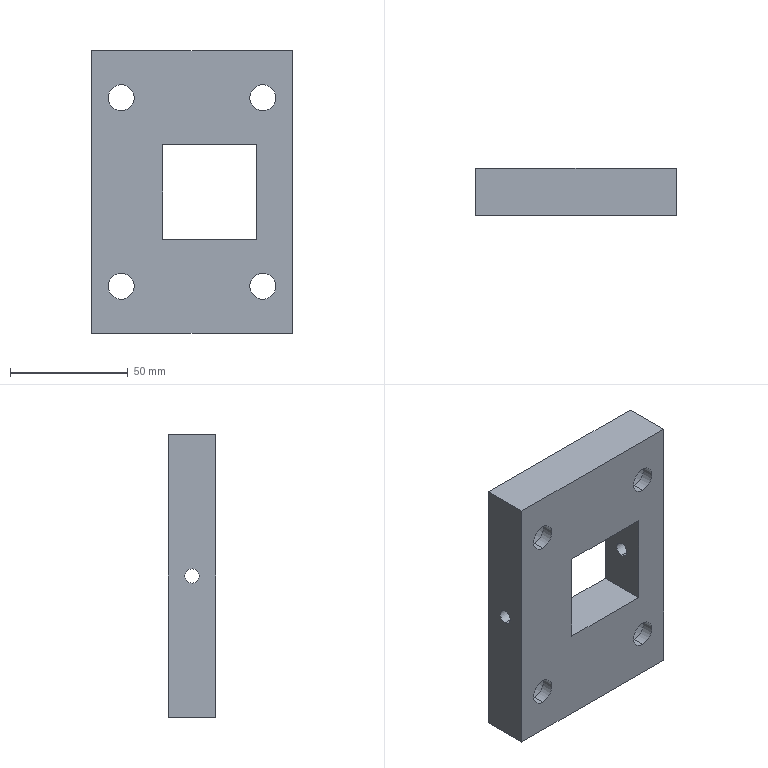Part | SolidWorks | features ICE 2, Extrusion 1 | 1 solid | 34 faces | box 85 x 20 x 120 mm | volume 147044 mm3 | cylinder 20 | plane 14 | commonest cylinder face diameters 11 x8 21.5 x8 6 x4
STEP:
#1=CARTESIAN_POINT('',(42.5,10.,-3.));
#2=VERTEX_POINT('',#1);
#3=CARTESIAN_POINT('',(42.5,10.,3.));
#4=VERTEX_POINT('',#3);
#5=CARTESIAN_POINT('',(42.5,10.,0.));
#6=DIRECTION('',(-1.,0.,0.));
#7=DIRECTION('',(0.,0.,1.));
#8=AXIS2_PLACEMENT_3D('',#5,#6,#7);
#9=CIRCLE('',#8,3.);
#10=EDGE_CURVE('',#2,#4,#9,.T.);
#11=ORIENTED_EDGE('',*,*,#10,.F.);
#12=CARTESIAN_POINT('',(27.5,10.,-3.));
#13=VERTEX_POINT('',#12);
#14=CARTESIAN_POINT('',(42.5,10.,-3.));
#15=DIRECTION('',(-1.,0.,0.));
#16=VECTOR('',#15,1000.);
#17=LINE('',#14,#16);
#18=EDGE_CURVE('',#2,#13,#17,.T.);
#19=ORIENTED_EDGE('',*,*,#18,.T.);
#20=CARTESIAN_POINT('',(27.5,10.,3.));
#21=VERTEX_POINT('',#20);
#22=CARTESIAN_POINT('',(27.5,10.,0.));
#23=DIRECTION('',(-1.,0.,0.));
#24=DIRECTION('',(0.,0.,1.));
#25=AXIS2_PLACEMENT_3D('',#22,#23,#24);
#26=CIRCLE('',#25,3.);
#27=EDGE_CURVE('',#13,#21,#26,.T.);
#28=ORIENTED_EDGE('',*,*,#27,.T.);
#29=CARTESIAN_POINT('',(42.5,10.,3.));
#30=DIRECTION('',(-1.,0.,0.));
#31=VECTOR('',#30,1000.);
#32=LINE('',#29,#31);
#33=EDGE_CURVE('',#4,#21,#32,.T.);
#34=ORIENTED_EDGE('',*,*,#33,.F.);
#35=EDGE_LOOP('',(#11,#19,#28,#34));
#36=FACE_OUTER_BOUND('',#35,.T.);
#37=CARTESIAN_POINT('',(42.5,10.,0.));
#38=DIRECTION('',(-1.,0.,0.));
#39=DIRECTION('',(0.,0.,1.));
#40=AXIS2_PLACEMENT_3D('',#37,#38,#39);
#41=CYLINDRICAL_SURFACE('',#40,3.);
#42=ADVANCED_FACE('',(#36),#41,.F.);
#43=CARTESIAN_POINT('',(-12.5,10.,3.));
#44=VERTEX_POINT('',#43);
#45=CARTESIAN_POINT('',(-12.5,10.,-3.));
#46=VERTEX_POINT('',#45);
#47=CARTESIAN_POINT('',(-12.5,10.,0.));
#48=DIRECTION('',(1.,0.,0.));
#49=DIRECTION('',(0.,0.,-1.));
#50=AXIS2_PLACEMENT_3D('',#47,#48,#49);
#51=CIRCLE('',#50,3.);
#52=EDGE_CURVE('',#44,#46,#51,.T.);
#53=ORIENTED_EDGE('',*,*,#52,.T.);
#54=CARTESIAN_POINT('',(-42.5,10.,-3.));
#55=VERTEX_POINT('',#54);
#56=CARTESIAN_POINT('',(42.5,10.,-3.));
#57=DIRECTION('',(-1.,0.,0.));
#58=VECTOR('',#57,1000.);
#59=LINE('',#56,#58);
#60=EDGE_CURVE('',#46,#55,#59,.T.);
#61=ORIENTED_EDGE('',*,*,#60,.T.);
#62=CARTESIAN_POINT('',(-42.5,10.,3.));
#63=VERTEX_POINT('',#62);
#64=CARTESIAN_POINT('',(-42.5,10.,0.));
#65=DIRECTION('',(-1.,0.,0.));
#66=DIRECTION('',(0.,0.,1.));
#67=AXIS2_PLACEMENT_3D('',#64,#65,#66);
#68=CIRCLE('',#67,3.);
#69=EDGE_CURVE('',#55,#63,#68,.T.);
#70=ORIENTED_EDGE('',*,*,#69,.T.);
#71=CARTESIAN_POINT('',(42.5,10.,3.));
#72=DIRECTION('',(-1.,0.,0.));
#73=VECTOR('',#72,1000.);
#74=LINE('',#71,#73);
#75=EDGE_CURVE('',#44,#63,#74,.T.);
#76=ORIENTED_EDGE('',*,*,#75,.F.);
#77=EDGE_LOOP('',(#53,#61,#70,#76));
#78=FACE_OUTER_BOUND('',#77,.T.);
#79=CARTESIAN_POINT('',(42.5,10.,0.));
#80=DIRECTION('',(-1.,0.,0.));
#81=DIRECTION('',(0.,0.,1.));
#82=AXIS2_PLACEMENT_3D('',#79,#80,#81);
#83=CYLINDRICAL_SURFACE('',#82,3.);
#84=ADVANCED_FACE('',(#78),#83,.F.);
#85=CARTESIAN_POINT('',(-30.,5.,-50.75));
#86=VERTEX_POINT('',#85);
#87=CARTESIAN_POINT('',(-30.,5.,-29.25));
#88=VERTEX_POINT('',#87);
#89=CARTESIAN_POINT('',(-30.,5.,-40.));
#90=DIRECTION('',(0.,1.,0.));
#91=DIRECTION('',(0.,0.,1.));
#92=AXIS2_PLACEMENT_3D('',#89,#90,#91);
#93=CIRCLE('',#92,10.75);
#94=EDGE_CURVE('',#86,#88,#93,.T.);
#95=ORIENTED_EDGE('',*,*,#94,.F.);
#96=CARTESIAN_POINT('',(-30.,20.,-50.75));
#97=VERTEX_POINT('',#96);
#98=CARTESIAN_POINT('',(-30.,5.,-50.75));
#99=DIRECTION('',(0.,1.,0.));
#100=VECTOR('',#99,1000.);
#101=LINE('',#98,#100);
#102=EDGE_CURVE('',#86,#97,#101,.T.);
#103=ORIENTED_EDGE('',*,*,#102,.T.);
#104=CARTESIAN_POINT('',(-30.,20.,-29.25));
#105=VERTEX_POINT('',#104);
#106=CARTESIAN_POINT('',(-30.,20.,-40.));
#107=DIRECTION('',(0.,1.,0.));
#108=DIRECTION('',(0.,0.,1.));
#109=AXIS2_PLACEMENT_3D('',#106,#107,#108);
#110=CIRCLE('',#109,10.75);
#111=EDGE_CURVE('',#97,#105,#110,.T.);
#112=ORIENTED_EDGE('',*,*,#111,.T.);
#113=CARTESIAN_POINT('',(-30.,5.,-29.25));
#114=DIRECTION('',(0.,1.,0.));
#115=VECTOR('',#114,1000.);
#116=LINE('',#113,#115);
#117=EDGE_CURVE('',#88,#105,#116,.T.);
#118=ORIENTED_EDGE('',*,*,#117,.F.);
#119=EDGE_LOOP('',(#95,#103,#112,#118));
#120=FACE_OUTER_BOUND('',#119,.T.);
#121=CARTESIAN_POINT('',(-30.,5.,-40.));
#122=DIRECTION('',(0.,1.,0.));
#123=DIRECTION('',(0.,0.,1.));
#124=AXIS2_PLACEMENT_3D('',#121,#122,#123);
#125=CYLINDRICAL_SURFACE('',#124,10.75);
#126=ADVANCED_FACE('',(#120),#125,.F.);
#127=CARTESIAN_POINT('',(30.,5.,-50.75));
#128=VERTEX_POINT('',#127);
#129=CARTESIAN_POINT('',(30.,5.,-29.25));
#130=VERTEX_POINT('',#129);
#131=CARTESIAN_POINT('',(30.,5.,-40.));
#132=DIRECTION('',(0.,1.,0.));
#133=DIRECTION('',(0.,0.,1.));
#134=AXIS2_PLACEMENT_3D('',#131,#132,#133);
#135=CIRCLE('',#134,10.75);
#136=EDGE_CURVE('',#128,#130,#135,.T.);
#137=ORIENTED_EDGE('',*,*,#136,.F.);
#138=CARTESIAN_POINT('',(30.,20.,-50.75));
#139=VERTEX_POINT('',#138);
#140=CARTESIAN_POINT('',(30.,5.,-50.75));
#141=DIRECTION('',(0.,1.,0.));
#142=VECTOR('',#141,1000.);
#143=LINE('',#140,#142);
#144=EDGE_CURVE('',#128,#139,#143,.T.);
#145=ORIENTED_EDGE('',*,*,#144,.T.);
#146=CARTESIAN_POINT('',(30.,20.,-29.25));
#147=VERTEX_POINT('',#146);
#148=CARTESIAN_POINT('',(30.,20.,-40.));
#149=DIRECTION('',(0.,1.,0.));
#150=DIRECTION('',(0.,0.,1.));
#151=AXIS2_PLACEMENT_3D('',#148,#149,#150);
#152=CIRCLE('',#151,10.75);
#153=EDGE_CURVE('',#139,#147,#152,.T.);
#154=ORIENTED_EDGE('',*,*,#153,.T.);
#155=CARTESIAN_POINT('',(30.,5.,-29.25));
#156=DIRECTION('',(0.,1.,0.));
#157=VECTOR('',#156,1000.);
#158=LINE('',#155,#157);
#159=EDGE_CURVE('',#130,#147,#158,.T.);
#160=ORIENTED_EDGE('',*,*,#159,.F.);
#161=EDGE_LOOP('',(#137,#145,#154,#160));
#162=FACE_OUTER_BOUND('',#161,.T.);
#163=CARTESIAN_POINT('',(30.,5.,-40.));
#164=DIRECTION('',(0.,1.,0.));
#165=DIRECTION('',(0.,0.,1.));
#166=AXIS2_PLACEMENT_3D('',#163,#164,#165);
#167=CYLINDRICAL_SURFACE('',#166,10.75);
#168=ADVANCED_FACE('',(#162),#167,.F.);
#169=CARTESIAN_POINT('',(30.,5.,29.25));
#170=VERTEX_POINT('',#169);
#171=CARTESIAN_POINT('',(30.,5.,50.75));
#172=VERTEX_POINT('',#171);
#173=CARTESIAN_POINT('',(30.,5.,40.));
#174=DIRECTION('',(0.,1.,0.));
#175=DIRECTION('',(0.,0.,1.));
#176=AXIS2_PLACEMENT_3D('',#173,#174,#175);
#177=CIRCLE('',#176,10.75);
#178=EDGE_CURVE('',#170,#172,#177,.T.);
#179=ORIENTED_EDGE('',*,*,#178,.F.);
#180=CARTESIAN_POINT('',(30.,20.,29.25));
#181=VERTEX_POINT('',#180);
#182=CARTESIAN_POINT('',(30.,5.,29.25));
#183=DIRECTION('',(0.,1.,0.));
#184=VECTOR('',#183,1000.);
#185=LINE('',#182,#184);
#186=EDGE_CURVE('',#170,#181,#185,.T.);
#187=ORIENTED_EDGE('',*,*,#186,.T.);
#188=CARTESIAN_POINT('',(30.,20.,50.75));
#189=VERTEX_POINT('',#188);
#190=CARTESIAN_POINT('',(30.,20.,40.));
#191=DIRECTION('',(0.,1.,0.));
#192=DIRECTION('',(0.,0.,1.));
#193=AXIS2_PLACEMENT_3D('',#190,#191,#192);
#194=CIRCLE('',#193,10.75);
#195=EDGE_CURVE('',#181,#189,#194,.T.);
#196=ORIENTED_EDGE('',*,*,#195,.T.);
#197=CARTESIAN_POINT('',(30.,5.,50.75));
#198=DIRECTION('',(0.,1.,0.));
#199=VECTOR('',#198,1000.);
#200=LINE('',#197,#199);
#201=EDGE_CURVE('',#172,#189,#200,.T.);
#202=ORIENTED_EDGE('',*,*,#201,.F.);
#203=EDGE_LOOP('',(#179,#187,#196,#202));
#204=FACE_OUTER_BOUND('',#203,.T.);
#205=CARTESIAN_POINT('',(30.,5.,40.));
#206=DIRECTION('',(0.,1.,0.));
#207=DIRECTION('',(0.,0.,1.));
#208=AXIS2_PLACEMENT_3D('',#205,#206,#207);
#209=CYLINDRICAL_SURFACE('',#208,10.75);
#210=ADVANCED_FACE('',(#204),#209,.F.);
#211=CARTESIAN_POINT('',(-30.,5.,29.25));
#212=VERTEX_POINT('',#211);
#213=CARTESIAN_POINT('',(-30.,5.,50.75));
#214=VERTEX_POINT('',#213);
#215=CARTESIAN_POINT('',(-30.,5.,40.));
#216=DIRECTION('',(0.,1.,0.));
#217=DIRECTION('',(0.,0.,1.));
#218=AXIS2_PLACEMENT_3D('',#215,#216,#217);
#219=CIRCLE('',#218,10.75);
#220=EDGE_CURVE('',#212,#214,#219,.T.);
#221=ORIENTED_EDGE('',*,*,#220,.F.);
#222=CARTESIAN_POINT('',(-30.,20.,29.25));
#223=VERTEX_POINT('',#222);
#224=CARTESIAN_POINT('',(-30.,5.,29.25));
#225=DIRECTION('',(0.,1.,0.));
#226=VECTOR('',#225,1000.);
#227=LINE('',#224,#226);
#228=EDGE_CURVE('',#212,#223,#227,.T.);
#229=ORIENTED_EDGE('',*,*,#228,.T.);
#230=CARTESIAN_POINT('',(-30.,20.,50.75));
#231=VERTEX_POINT('',#230);
#232=CARTESIAN_POINT('',(-30.,20.,40.));
#233=DIRECTION('',(0.,1.,0.));
#234=DIRECTION('',(0.,0.,1.));
#235=AXIS2_PLACEMENT_3D('',#232,#233,#234);
#236=CIRCLE('',#235,10.75);
#237=EDGE_CURVE('',#223,#231,#236,.T.);
#238=ORIENTED_EDGE('',*,*,#237,.T.);
#239=CARTESIAN_POINT('',(-30.,5.,50.75));
#240=DIRECTION('',(0.,1.,0.));
#241=VECTOR('',#240,1000.);
#242=LINE('',#239,#241);
#243=EDGE_CURVE('',#214,#231,#242,.T.);
#244=ORIENTED_EDGE('',*,*,#243,.F.);
#245=EDGE_LOOP('',(#221,#229,#238,#244));
#246=FACE_OUTER_BOUND('',#245,.T.);
#247=CARTESIAN_POINT('',(-30.,5.,40.));
#248=DIRECTION('',(0.,1.,0.));
#249=DIRECTION('',(0.,0.,1.));
#250=AXIS2_PLACEMENT_3D('',#247,#248,#249);
#251=CYLINDRICAL_SURFACE('',#250,10.75);
#252=ADVANCED_FACE('',(#246),#251,.F.);
#253=CARTESIAN_POINT('',(-30.,5.,34.5));
#254=VERTEX_POINT('',#253);
#255=CARTESIAN_POINT('',(-30.,5.,45.5));
#256=VERTEX_POINT('',#255);
#257=CARTESIAN_POINT('',(-30.,5.,40.));
#258=DIRECTION('',(0.,1.,0.));
#259=DIRECTION('',(0.,0.,1.));
#260=AXIS2_PLACEMENT_3D('',#257,#258,#259);
#261=CIRCLE('',#260,5.5);
#262=EDGE_CURVE('',#254,#256,#261,.T.);
#263=ORIENTED_EDGE('',*,*,#262,.T.);
#264=CARTESIAN_POINT('',(-30.,0.,45.5));
#265=VERTEX_POINT('',#264);
#266=CARTESIAN_POINT('',(-30.,20.,45.5));
#267=DIRECTION('',(0.,-1.,0.));
#268=VECTOR('',#267,1000.);
#269=LINE('',#266,#268);
#270=EDGE_CURVE('',#256,#265,#269,.T.);
#271=ORIENTED_EDGE('',*,*,#270,.T.);
#272=CARTESIAN_POINT('',(-30.,0.,34.5));
#273=VERTEX_POINT('',#272);
#274=CARTESIAN_POINT('',(-30.,0.,40.));
#275=DIRECTION('',(0.,1.,0.));
#276=DIRECTION('',(0.,0.,1.));
#277=AXIS2_PLACEMENT_3D('',#274,#275,#276);
#278=CIRCLE('',#277,5.5);
#279=EDGE_CURVE('',#273,#265,#278,.T.);
#280=ORIENTED_EDGE('',*,*,#279,.F.);
#281=CARTESIAN_POINT('',(-30.,20.,34.5));
#282=DIRECTION('',(0.,-1.,0.));
#283=VECTOR('',#282,1000.);
#284=LINE('',#281,#283);
#285=EDGE_CURVE('',#254,#273,#284,.T.);
#286=ORIENTED_EDGE('',*,*,#285,.F.);
#287=EDGE_LOOP('',(#263,#271,#280,#286));
#288=FACE_OUTER_BOUND('',#287,.T.);
#289=CARTESIAN_POINT('',(-30.,20.,40.));
#290=DIRECTION('',(0.,-1.,0.));
#291=DIRECTION('',(0.,0.,-1.));
#292=AXIS2_PLACEMENT_3D('',#289,#290,#291);
#293=CYLINDRICAL_SURFACE('',#292,5.5);
#294=ADVANCED_FACE('',(#288),#293,.F.);
#295=CARTESIAN_POINT('',(30.,5.,34.5));
#296=VERTEX_POINT('',#295);
#297=CARTESIAN_POINT('',(30.,5.,45.5));
#298=VERTEX_POINT('',#297);
#299=CARTESIAN_POINT('',(30.,5.,40.));
#300=DIRECTION('',(0.,1.,0.));
#301=DIRECTION('',(0.,0.,1.));
#302=AXIS2_PLACEMENT_3D('',#299,#300,#301);
#303=CIRCLE('',#302,5.5);
#304=EDGE_CURVE('',#296,#298,#303,.T.);
#305=ORIENTED_EDGE('',*,*,#304,.T.);
#306=CARTESIAN_POINT('',(30.,0.,45.5));
#307=VERTEX_POINT('',#306);
#308=CARTESIAN_POINT('',(30.,20.,45.5));
#309=DIRECTION('',(0.,-1.,0.));
#310=VECTOR('',#309,1000.);
#311=LINE('',#308,#310);
#312=EDGE_CURVE('',#298,#307,#311,.T.);
#313=ORIENTED_EDGE('',*,*,#312,.T.);
#314=CARTESIAN_POINT('',(30.,0.,34.5));
#315=VERTEX_POINT('',#314);
#316=CARTESIAN_POINT('',(30.,0.,40.));
#317=DIRECTION('',(0.,1.,0.));
#318=DIRECTION('',(0.,0.,1.));
#319=AXIS2_PLACEMENT_3D('',#316,#317,#318);
#320=CIRCLE('',#319,5.5);
#321=EDGE_CURVE('',#315,#307,#320,.T.);
#322=ORIENTED_EDGE('',*,*,#321,.F.);
#323=CARTESIAN_POINT('',(30.,20.,34.5));
#324=DIRECTION('',(0.,-1.,0.));
#325=VECTOR('',#324,1000.);
#326=LINE('',#323,#325);
#327=EDGE_CURVE('',#296,#315,#326,.T.);
#328=ORIENTED_EDGE('',*,*,#327,.F.);
#329=EDGE_LOOP('',(#305,#313,#322,#328));
#330=FACE_OUTER_BOUND('',#329,.T.);
#331=CARTESIAN_POINT('',(30.,20.,40.));
#332=DIRECTION('',(0.,-1.,0.));
#333=DIRECTION('',(0.,0.,-1.));
#334=AXIS2_PLACEMENT_3D('',#331,#332,#333);
#335=CYLINDRICAL_SURFACE('',#334,5.5);
#336=ADVANCED_FACE('',(#330),#335,.F.);
#337=CARTESIAN_POINT('',(30.,5.,-45.5));
#338=VERTEX_POINT('',#337);
#339=CARTESIAN_POINT('',(30.,5.,-34.5));
#340=VERTEX_POINT('',#339);
#341=CARTESIAN_POINT('',(30.,5.,-40.));
#342=DIRECTION('',(0.,1.,0.));
#343=DIRECTION('',(0.,0.,1.));
#344=AXIS2_PLACEMENT_3D('',#341,#342,#343);
#345=CIRCLE('',#344,5.5);
#346=EDGE_CURVE('',#338,#340,#345,.T.);
#347=ORIENTED_EDGE('',*,*,#346,.T.);
#348=CARTESIAN_POINT('',(30.,0.,-34.5));
#349=VERTEX_POINT('',#348);
#350=CARTESIAN_POINT('',(30.,20.,-34.5));
#351=DIRECTION('',(0.,-1.,0.));
#352=VECTOR('',#351,1000.);
#353=LINE('',#350,#352);
#354=EDGE_CURVE('',#340,#349,#353,.T.);
#355=ORIENTED_EDGE('',*,*,#354,.T.);
#356=CARTESIAN_POINT('',(30.,0.,-45.5));
#357=VERTEX_POINT('',#356);
#358=CARTESIAN_POINT('',(30.,0.,-40.));
#359=DIRECTION('',(0.,1.,0.));
#360=DIRECTION('',(0.,0.,1.));
#361=AXIS2_PLACEMENT_3D('',#358,#359,#360);
#362=CIRCLE('',#361,5.5);
#363=EDGE_CURVE('',#357,#349,#362,.T.);
#364=ORIENTED_EDGE('',*,*,#363,.F.);
#365=CARTESIAN_POINT('',(30.,20.,-45.5));
#366=DIRECTION('',(0.,-1.,0.));
#367=VECTOR('',#366,1000.);
#368=LINE('',#365,#367);
#369=EDGE_CURVE('',#338,#357,#368,.T.);
#370=ORIENTED_EDGE('',*,*,#369,.F.);
#371=EDGE_LOOP('',(#347,#355,#364,#370));
#372=FACE_OUTER_BOUND('',#371,.T.);
#373=CARTESIAN_POINT('',(30.,20.,-40.));
#374=DIRECTION('',(0.,-1.,0.));
#375=DIRECTION('',(0.,0.,-1.));
#376=AXIS2_PLACEMENT_3D('',#373,#374,#375);
#377=CYLINDRICAL_SURFACE('',#376,5.5);
#378=ADVANCED_FACE('',(#372),#377,.F.);
#379=CARTESIAN_POINT('',(-30.,5.,-45.5));
#380=VERTEX_POINT('',#379);
#381=CARTESIAN_POINT('',(-30.,5.,-34.5));
#382=VERTEX_POINT('',#381);
#383=CARTESIAN_POINT('',(-30.,5.,-40.));
#384=DIRECTION('',(0.,1.,0.));
#385=DIRECTION('',(0.,0.,1.));
#386=AXIS2_PLACEMENT_3D('',#383,#384,#385);
#387=CIRCLE('',#386,5.5);
#388=EDGE_CURVE('',#380,#382,#387,.T.);
#389=ORIENTED_EDGE('',*,*,#388,.T.);
#390=CARTESIAN_POINT('',(-30.,0.,-34.5));
#391=VERTEX_POINT('',#390);
#392=CARTESIAN_POINT('',(-30.,20.,-34.5));
#393=DIRECTION('',(0.,-1.,0.));
#394=VECTOR('',#393,1000.);
#395=LINE('',#392,#394);
#396=EDGE_CURVE('',#382,#391,#395,.T.);
#397=ORIENTED_EDGE('',*,*,#396,.T.);
#398=CARTESIAN_POINT('',(-30.,0.,-45.5));
#399=VERTEX_POINT('',#398);
#400=CARTESIAN_POINT('',(-30.,0.,-40.));
#401=DIRECTION('',(0.,1.,0.));
#402=DIRECTION('',(0.,0.,1.));
#403=AXIS2_PLACEMENT_3D('',#400,#401,#402);
#404=CIRCLE('',#403,5.5);
#405=EDGE_CURVE('',#399,#391,#404,.T.);
#406=ORIENTED_EDGE('',*,*,#405,.F.);
#407=CARTESIAN_POINT('',(-30.,20.,-45.5));
#408=DIRECTION('',(0.,-1.,0.));
#409=VECTOR('',#408,1000.);
#410=LINE('',#407,#409);
#411=EDGE_CURVE('',#380,#399,#410,.T.);
#412=ORIENTED_EDGE('',*,*,#411,.F.);
#413=EDGE_LOOP('',(#389,#397,#406,#412));
#414=FACE_OUTER_BOUND('',#413,.T.);
#415=CARTESIAN_POINT('',(-30.,20.,-40.));
#416=DIRECTION('',(0.,-1.,0.));
#417=DIRECTION('',(0.,0.,-1.));
#418=AXIS2_PLACEMENT_3D('',#415,#416,#417);
#419=CYLINDRICAL_SURFACE('',#418,5.5);
#420=ADVANCED_FACE('',(#414),#419,.F.);
#421=ORIENTED_EDGE('',*,*,#396,.F.);
#422=CARTESIAN_POINT('',(-30.,5.,-40.));
#423=DIRECTION('',(0.,1.,0.));
#424=DIRECTION('',(0.,0.,1.));
#425=AXIS2_PLACEMENT_3D('',#422,#423,#424);
#426=CIRCLE('',#425,5.5);
#427=EDGE_CURVE('',#382,#380,#426,.T.);
#428=ORIENTED_EDGE('',*,*,#427,.T.);
#429=ORIENTED_EDGE('',*,*,#411,.T.);
#430=CARTESIAN_POINT('',(-30.,0.,-40.));
#431=DIRECTION('',(0.,1.,0.));
#432=DIRECTION('',(0.,0.,1.));
#433=AXIS2_PLACEMENT_3D('',#430,#431,#432);
#434=CIRCLE('',#433,5.5);
#435=EDGE_CURVE('',#391,#399,#434,.T.);
#436=ORIENTED_EDGE('',*,*,#435,.F.);
#437=EDGE_LOOP('',(#421,#428,#429,#436));
#438=FACE_OUTER_BOUND('',#437,.T.);
#439=CARTESIAN_POINT('',(-30.,20.,-40.));
#440=DIRECTION('',(0.,-1.,0.));
#441=DIRECTION('',(0.,0.,-1.));
#442=AXIS2_PLACEMENT_3D('',#439,#440,#441);
#443=CYLINDRICAL_SURFACE('',#442,5.5);
#444=ADVANCED_FACE('',(#438),#443,.F.);
#445=ORIENTED_EDGE('',*,*,#354,.F.);
#446=CARTESIAN_POINT('',(30.,5.,-40.));
#447=DIRECTION('',(0.,1.,0.));
#448=DIRECTION('',(0.,0.,1.));
#449=AXIS2_PLACEMENT_3D('',#446,#447,#448);
#450=CIRCLE('',#449,5.5);
#451=EDGE_CURVE('',#340,#338,#450,.T.);
#452=ORIENTED_EDGE('',*,*,#451,.T.);
#453=ORIENTED_EDGE('',*,*,#369,.T.);
#454=CARTESIAN_POINT('',(30.,0.,-40.));
#455=DIRECTION('',(0.,1.,0.));
#456=DIRECTION('',(0.,0.,1.));
#457=AXIS2_PLACEMENT_3D('',#454,#455,#456);
#458=CIRCLE('',#457,5.5);
#459=EDGE_CURVE('',#349,#357,#458,.T.);
#460=ORIENTED_EDGE('',*,*,#459,.F.);
#461=EDGE_LOOP('',(#445,#452,#453,#460));
#462=FACE_OUTER_BOUND('',#461,.T.);
#463=CARTESIAN_POINT('',(30.,20.,-40.));
#464=DIRECTION('',(0.,-1.,0.));
#465=DIRECTION('',(0.,0.,-1.));
#466=AXIS2_PLACEMENT_3D('',#463,#464,#465);
#467=CYLINDRICAL_SURFACE('',#466,5.5);
#468=ADVANCED_FACE('',(#462),#467,.F.);
#469=ORIENTED_EDGE('',*,*,#312,.F.);
#470=CARTESIAN_POINT('',(30.,5.,40.));
#471=DIRECTION('',(0.,1.,0.));
#472=DIRECTION('',(0.,0.,1.));
#473=AXIS2_PLACEMENT_3D('',#470,#471,#472);
#474=CIRCLE('',#473,5.5);
#475=EDGE_CURVE('',#298,#296,#474,.T.);
#476=ORIENTED_EDGE('',*,*,#475,.T.);
#477=ORIENTED_EDGE('',*,*,#327,.T.);
#478=CARTESIAN_POINT('',(30.,0.,40.));
#479=DIRECTION('',(0.,1.,0.));
#480=DIRECTION('',(0.,0.,1.));
#481=AXIS2_PLACEMENT_3D('',#478,#479,#480);
#482=CIRCLE('',#481,5.5);
#483=EDGE_CURVE('',#307,#315,#482,.T.);
#484=ORIENTED_EDGE('',*,*,#483,.F.);
#485=EDGE_LOOP('',(#469,#476,#477,#484));
#486=FACE_OUTER_BOUND('',#485,.T.);
#487=CARTESIAN_POINT('',(30.,20.,40.));
#488=DIRECTION('',(0.,-1.,0.));
#489=DIRECTION('',(0.,0.,-1.));
#490=AXIS2_PLACEMENT_3D('',#487,#488,#489);
#491=CYLINDRICAL_SURFACE('',#490,5.5);
#492=ADVANCED_FACE('',(#486),#491,.F.);
#493=ORIENTED_EDGE('',*,*,#270,.F.);
#494=CARTESIAN_POINT('',(-30.,5.,40.));
#495=DIRECTION('',(0.,1.,0.));
#496=DIRECTION('',(0.,0.,1.));
#497=AXIS2_PLACEMENT_3D('',#494,#495,#496);
#498=CIRCLE('',#497,5.5);
#499=EDGE_CURVE('',#256,#254,#498,.T.);
#500=ORIENTED_EDGE('',*,*,#499,.T.);
#501=ORIENTED_EDGE('',*,*,#285,.T.);
#502=CARTESIAN_POINT('',(-30.,0.,40.));
#503=DIRECTION('',(0.,1.,0.));
#504=DIRECTION('',(0.,0.,1.));
#505=AXIS2_PLACEMENT_3D('',#502,#503,#504);
#506=CIRCLE('',#505,5.5);
#507=EDGE_CURVE('',#265,#273,#506,.T.);
#508=ORIENTED_EDGE('',*,*,#507,.F.);
#509=EDGE_LOOP('',(#493,#500,#501,#508));
#510=FACE_OUTER_BOUND('',#509,.T.);
#511=CARTESIAN_POINT('',(-30.,20.,40.));
#512=DIRECTION('',(0.,-1.,0.));
#513=DIRECTION('',(0.,0.,-1.));
#514=AXIS2_PLACEMENT_3D('',#511,#512,#513);
#515=CYLINDRICAL_SURFACE('',#514,5.5);
#516=ADVANCED_FACE('',(#510),#515,.F.);
#517=CARTESIAN_POINT('',(30.,20.,40.));
#518=DIRECTION('',(0.,1.,0.));
#519=DIRECTION('',(0.,0.,1.));
#520=AXIS2_PLACEMENT_3D('',#517,#518,#519);
#521=CIRCLE('',#520,10.75);
#522=EDGE_CURVE('',#189,#181,#521,.T.);
#523=ORIENTED_EDGE('',*,*,#522,.F.);
#524=ORIENTED_EDGE('',*,*,#195,.F.);
#525=EDGE_LOOP('',(#523,#524));
#526=FACE_BOUND('',#525,.T.);
#527=CARTESIAN_POINT('',(-30.,20.,40.));
#528=DIRECTION('',(0.,1.,0.));
#529=DIRECTION('',(0.,0.,1.));
#530=AXIS2_PLACEMENT_3D('',#527,#528,#529);
#531=CIRCLE('',#530,10.75);
#532=EDGE_CURVE('',#231,#223,#531,.T.);
#533=ORIENTED_EDGE('',*,*,#532,.F.);
#534=ORIENTED_EDGE('',*,*,#237,.F.);
#535=EDGE_LOOP('',(#533,#534));
#536=FACE_BOUND('',#535,.T.);
#537=CARTESIAN_POINT('',(-30.,20.,-40.));
#538=DIRECTION('',(0.,1.,0.));
#539=DIRECTION('',(0.,0.,1.));
#540=AXIS2_PLACEMENT_3D('',#537,#538,#539);
#541=CIRCLE('',#540,10.75);
#542=EDGE_CURVE('',#105,#97,#541,.T.);
#543=ORIENTED_EDGE('',*,*,#542,.F.);
#544=ORIENTED_EDGE('',*,*,#111,.F.);
#545=EDGE_LOOP('',(#543,#544));
#546=FACE_BOUND('',#545,.T.);
#547=CARTESIAN_POINT('',(30.,20.,-40.));
#548=DIRECTION('',(0.,1.,0.));
#549=DIRECTION('',(0.,0.,1.));
#550=AXIS2_PLACEMENT_3D('',#547,#548,#549);
#551=CIRCLE('',#550,10.75);
#552=EDGE_CURVE('',#147,#139,#551,.T.);
#553=ORIENTED_EDGE('',*,*,#552,.F.);
#554=ORIENTED_EDGE('',*,*,#153,.F.);
#555=EDGE_LOOP('',(#553,#554));
#556=FACE_BOUND('',#555,.T.);
#557=CARTESIAN_POINT('',(42.5,20.,60.));
#558=VERTEX_POINT('',#557);
#559=CARTESIAN_POINT('',(42.5,20.,-60.));
#560=VERTEX_POINT('',#559);
#561=CARTESIAN_POINT('',(42.5,20.,60.));
#562=DIRECTION('',(0.,0.,-1.));
#563=VECTOR('',#562,1000.);
#564=LINE('',#561,#563);
#565=EDGE_CURVE('',#558,#560,#564,.T.);
#566=ORIENTED_EDGE('',*,*,#565,.T.);
#567=CARTESIAN_POINT('',(-42.5,20.,-60.));
#568=VERTEX_POINT('',#567);
#569=CARTESIAN_POINT('',(-42.5,20.,-60.));
#570=DIRECTION('',(-1.,0.,0.));
#571=VECTOR('',#570,1000.);
#572=LINE('',#569,#571);
#573=EDGE_CURVE('',#560,#568,#572,.T.);
#574=ORIENTED_EDGE('',*,*,#573,.T.);
#575=CARTESIAN_POINT('',(-42.5,20.,60.));
#576=VERTEX_POINT('',#575);
#577=CARTESIAN_POINT('',(-42.5,20.,60.));
#578=DIRECTION('',(0.,0.,1.));
#579=VECTOR('',#578,1000.);
#580=LINE('',#577,#579);
#581=EDGE_CURVE('',#568,#576,#580,.T.);
#582=ORIENTED_EDGE('',*,*,#581,.T.);
#583=CARTESIAN_POINT('',(-42.5,20.,60.));
#584=DIRECTION('',(1.,0.,0.));
#585=VECTOR('',#584,1000.);
#586=LINE('',#583,#585);
#587=EDGE_CURVE('',#576,#558,#586,.T.);
#588=ORIENTED_EDGE('',*,*,#587,.T.);
#589=EDGE_LOOP('',(#566,#574,#582,#588));
#590=FACE_OUTER_BOUND('',#589,.T.);
#591=CARTESIAN_POINT('',(27.5,20.,20.));
#592=VERTEX_POINT('',#591);
#593=CARTESIAN_POINT('',(27.5,20.,-20.));
#594=VERTEX_POINT('',#593);
#595=CARTESIAN_POINT('',(27.5,20.,20.));
#596=DIRECTION('',(0.,0.,-1.));
#597=VECTOR('',#596,1000.);
#598=LINE('',#595,#597);
#599=EDGE_CURVE('',#592,#594,#598,.T.);
#600=ORIENTED_EDGE('',*,*,#599,.F.);
#601=CARTESIAN_POINT('',(-12.5,20.,20.));
#602=VERTEX_POINT('',#601);
#603=CARTESIAN_POINT('',(-12.5,20.,20.));
#604=DIRECTION('',(1.,0.,0.));
#605=VECTOR('',#604,1000.);
#606=LINE('',#603,#605);
#607=EDGE_CURVE('',#602,#592,#606,.T.);
#608=ORIENTED_EDGE('',*,*,#607,.F.);
#609=CARTESIAN_POINT('',(-12.5,20.,-20.));
#610=VERTEX_POINT('',#609);
#611=CARTESIAN_POINT('',(-12.5,20.,20.));
#612=DIRECTION('',(0.,0.,1.));
#613=VECTOR('',#612,1000.);
#614=LINE('',#611,#613);
#615=EDGE_CURVE('',#610,#602,#614,.T.);
#616=ORIENTED_EDGE('',*,*,#615,.F.);
#617=CARTESIAN_POINT('',(-12.5,20.,-20.));
#618=DIRECTION('',(-1.,0.,0.));
#619=VECTOR('',#618,1000.);
#620=LINE('',#617,#619);
#621=EDGE_CURVE('',#594,#610,#620,.T.);
#622=ORIENTED_EDGE('',*,*,#621,.F.);
#623=EDGE_LOOP('',(#600,#608,#616,#622));
#624=FACE_BOUND('',#623,.T.);
#625=CARTESIAN_POINT('',(0.,20.,0.));
#626=DIRECTION('',(0.,-1.,0.));
#627=DIRECTION('',(0.,0.,-1.));
#628=AXIS2_PLACEMENT_3D('',#625,#626,#627);
#629=PLANE('',#628);
#630=ADVANCED_FACE('',(#526,#536,#546,#556,#590,#624),#629,.F.);
#631=ORIENTED_EDGE('',*,*,#321,.T.);
#632=ORIENTED_EDGE('',*,*,#483,.T.);
#633=EDGE_LOOP('',(#631,#632));
#634=FACE_BOUND('',#633,.T.);
#635=ORIENTED_EDGE('',*,*,#405,.T.);
#636=ORIENTED_EDGE('',*,*,#435,.T.);
#637=EDGE_LOOP('',(#635,#636));
#638=FACE_BOUND('',#637,.T.);
#639=CARTESIAN_POINT('',(42.5,0.,60.));
#640=VERTEX_POINT('',#639);
#641=CARTESIAN_POINT('',(42.5,0.,-60.));
#642=VERTEX_POINT('',#641);
#643=CARTESIAN_POINT('',(42.5,0.,60.));
#644=DIRECTION('',(0.,0.,-1.));
#645=VECTOR('',#644,1000.);
#646=LINE('',#643,#645);
#647=EDGE_CURVE('',#640,#642,#646,.T.);
#648=ORIENTED_EDGE('',*,*,#647,.F.);
#649=CARTESIAN_POINT('',(-42.5,0.,60.));
#650=VERTEX_POINT('',#649);
#651=CARTESIAN_POINT('',(-42.5,0.,60.));
#652=DIRECTION('',(1.,0.,0.));
#653=VECTOR('',#652,1000.);
#654=LINE('',#651,#653);
#655=EDGE_CURVE('',#650,#640,#654,.T.);
#656=ORIENTED_EDGE('',*,*,#655,.F.);
#657=CARTESIAN_POINT('',(-42.5,0.,-60.));
#658=VERTEX_POINT('',#657);
#659=CARTESIAN_POINT('',(-42.5,0.,60.));
#660=DIRECTION('',(0.,0.,1.));
#661=VECTOR('',#660,1000.);
#662=LINE('',#659,#661);
#663=EDGE_CURVE('',#658,#650,#662,.T.);
#664=ORIENTED_EDGE('',*,*,#663,.F.);
#665=CARTESIAN_POINT('',(-42.5,0.,-60.));
#666=DIRECTION('',(-1.,0.,0.));
#667=VECTOR('',#666,1000.);
#668=LINE('',#665,#667);
#669=EDGE_CURVE('',#642,#658,#668,.T.);
#670=ORIENTED_EDGE('',*,*,#669,.F.);
#671=EDGE_LOOP('',(#648,#656,#664,#670));
#672=FACE_OUTER_BOUND('',#671,.T.);
#673=ORIENTED_EDGE('',*,*,#363,.T.);
#674=ORIENTED_EDGE('',*,*,#459,.T.);
#675=EDGE_LOOP('',(#673,#674));
#676=FACE_BOUND('',#675,.T.);
#677=ORIENTED_EDGE('',*,*,#279,.T.);
#678=ORIENTED_EDGE('',*,*,#507,.T.);
#679=EDGE_LOOP('',(#677,#678));
#680=FACE_BOUND('',#679,.T.);
#681=CARTESIAN_POINT('',(-12.5,0.,20.));
#682=VERTEX_POINT('',#681);
#683=CARTESIAN_POINT('',(27.5,0.,20.));
#684=VERTEX_POINT('',#683);
#685=CARTESIAN_POINT('',(-12.5,0.,20.));
#686=DIRECTION('',(1.,0.,0.));
#687=VECTOR('',#686,1000.);
#688=LINE('',#685,#687);
#689=EDGE_CURVE('',#682,#684,#688,.T.);
#690=ORIENTED_EDGE('',*,*,#689,.T.);
#691=CARTESIAN_POINT('',(27.5,0.,-20.));
#692=VERTEX_POINT('',#691);
#693=CARTESIAN_POINT('',(27.5,0.,20.));
#694=DIRECTION('',(0.,0.,-1.));
#695=VECTOR('',#694,1000.);
#696=LINE('',#693,#695);
#697=EDGE_CURVE('',#684,#692,#696,.T.);
#698=ORIENTED_EDGE('',*,*,#697,.T.);
#699=CARTESIAN_POINT('',(-12.5,0.,-20.));
#700=VERTEX_POINT('',#699);
#701=CARTESIAN_POINT('',(-12.5,0.,-20.));
#702=DIRECTION('',(-1.,0.,0.));
#703=VECTOR('',#702,1000.);
#704=LINE('',#701,#703);
#705=EDGE_CURVE('',#692,#700,#704,.T.);
#706=ORIENTED_EDGE('',*,*,#705,.T.);
#707=CARTESIAN_POINT('',(-12.5,0.,20.));
#708=DIRECTION('',(0.,0.,1.));
#709=VECTOR('',#708,1000.);
#710=LINE('',#707,#709);
#711=EDGE_CURVE('',#700,#682,#710,.T.);
#712=ORIENTED_EDGE('',*,*,#711,.T.);
#713=EDGE_LOOP('',(#690,#698,#706,#712));
#714=FACE_BOUND('',#713,.T.);
#715=CARTESIAN_POINT('',(0.,0.,0.));
#716=DIRECTION('',(0.,-1.,0.));
#717=DIRECTION('',(0.,0.,-1.));
#718=AXIS2_PLACEMENT_3D('',#715,#716,#717);
#719=PLANE('',#718);
#720=ADVANCED_FACE('',(#634,#638,#672,#676,#680,#714),#719,.T.);
#721=CARTESIAN_POINT('',(42.5,10.,0.));
#722=DIRECTION('',(-1.,0.,0.));
#723=DIRECTION('',(0.,0.,1.));
#724=AXIS2_PLACEMENT_3D('',#721,#722,#723);
#725=CIRCLE('',#724,3.);
#726=EDGE_CURVE('',#4,#2,#725,.T.);
#727=ORIENTED_EDGE('',*,*,#726,.T.);
#728=ORIENTED_EDGE('',*,*,#10,.T.);
#729=EDGE_LOOP('',(#727,#728));
#730=FACE_BOUND('',#729,.T.);
#731=ORIENTED_EDGE('',*,*,#647,.T.);
#732=CARTESIAN_POINT('',(42.5,20.,-60.));
#733=DIRECTION('',(0.,-1.,0.));
#734=VECTOR('',#733,1000.);
#735=LINE('',#732,#734);
#736=EDGE_CURVE('',#560,#642,#735,.T.);
#737=ORIENTED_EDGE('',*,*,#736,.F.);
#738=ORIENTED_EDGE('',*,*,#565,.F.);
#739=CARTESIAN_POINT('',(42.5,20.,60.));
#740=DIRECTION('',(0.,-1.,0.));
#741=VECTOR('',#740,1000.);
#742=LINE('',#739,#741);
#743=EDGE_CURVE('',#558,#640,#742,.T.);
#744=ORIENTED_EDGE('',*,*,#743,.T.);
#745=EDGE_LOOP('',(#731,#737,#738,#744));
#746=FACE_OUTER_BOUND('',#745,.T.);
#747=CARTESIAN_POINT('',(42.5,20.,60.));
#748=DIRECTION('',(-1.,0.,0.));
#749=DIRECTION('',(0.,0.,1.));
#750=AXIS2_PLACEMENT_3D('',#747,#748,#749);
#751=PLANE('',#750);
#752=ADVANCED_FACE('',(#730,#746),#751,.F.);
#753=ORIENTED_EDGE('',*,*,#669,.T.);
#754=CARTESIAN_POINT('',(-42.5,20.,-60.));
#755=DIRECTION('',(0.,-1.,0.));
#756=VECTOR('',#755,1000.);
#757=LINE('',#754,#756);
#758=EDGE_CURVE('',#568,#658,#757,.T.);
#759=ORIENTED_EDGE('',*,*,#758,.F.);
#760=ORIENTED_EDGE('',*,*,#573,.F.);
#761=ORIENTED_EDGE('',*,*,#736,.T.);
#762=EDGE_LOOP('',(#753,#759,#760,#761));
#763=FACE_OUTER_BOUND('',#762,.T.);
#764=CARTESIAN_POINT('',(-42.5,20.,-60.));
#765=DIRECTION('',(0.,0.,1.));
#766=DIRECTION('',(1.,0.,0.));
#767=AXIS2_PLACEMENT_3D('',#764,#765,#766);
#768=PLANE('',#767);
#769=ADVANCED_FACE('',(#763),#768,.F.);
#770=CARTESIAN_POINT('',(-42.5,10.,0.));
#771=DIRECTION('',(-1.,0.,0.));
#772=DIRECTION('',(0.,0.,1.));
#773=AXIS2_PLACEMENT_3D('',#770,#771,#772);
#774=CIRCLE('',#773,3.);
#775=EDGE_CURVE('',#63,#55,#774,.T.);
#776=ORIENTED_EDGE('',*,*,#775,.F.);
#777=ORIENTED_EDGE('',*,*,#69,.F.);
#778=EDGE_LOOP('',(#776,#777));
#779=FACE_BOUND('',#778,.T.);
#780=ORIENTED_EDGE('',*,*,#663,.T.);
#781=CARTESIAN_POINT('',(-42.5,20.,60.));
#782=DIRECTION('',(0.,-1.,0.));
#783=VECTOR('',#782,1000.);
#784=LINE('',#781,#783);
#785=EDGE_CURVE('',#576,#650,#784,.T.);
#786=ORIENTED_EDGE('',*,*,#785,.F.);
#787=ORIENTED_EDGE('',*,*,#581,.F.);
#788=ORIENTED_EDGE('',*,*,#758,.T.);
#789=EDGE_LOOP('',(#780,#786,#787,#788));
#790=FACE_OUTER_BOUND('',#789,.T.);
#791=CARTESIAN_POINT('',(-42.5,20.,60.));
#792=DIRECTION('',(1.,0.,0.));
#793=DIRECTION('',(0.,0.,-1.));
#794=AXIS2_PLACEMENT_3D('',#791,#792,#793);
#795=PLANE('',#794);
#796=ADVANCED_FACE('',(#779,#790),#795,.F.);
#797=ORIENTED_EDGE('',*,*,#655,.T.);
#798=ORIENTED_EDGE('',*,*,#743,.F.);
#799=ORIENTED_EDGE('',*,*,#587,.F.);
#800=ORIENTED_EDGE('',*,*,#785,.T.);
#801=EDGE_LOOP('',(#797,#798,#799,#800));
#802=FACE_OUTER_BOUND('',#801,.T.);
#803=CARTESIAN_POINT('',(-42.5,20.,60.));
#804=DIRECTION('',(0.,0.,-1.));
#805=DIRECTION('',(-1.,0.,0.));
#806=AXIS2_PLACEMENT_3D('',#803,#804,#805);
#807=PLANE('',#806);
#808=ADVANCED_FACE('',(#802),#807,.F.);
#809=CARTESIAN_POINT('',(27.5,10.,0.));
#810=DIRECTION('',(-1.,0.,0.));
#811=DIRECTION('',(0.,0.,1.));
#812=AXIS2_PLACEMENT_3D('',#809,#810,#811);
#813=CIRCLE('',#812,3.);
#814=EDGE_CURVE('',#21,#13,#813,.T.);
#815=ORIENTED_EDGE('',*,*,#814,.F.);
#816=ORIENTED_EDGE('',*,*,#27,.F.);
#817=EDGE_LOOP('',(#815,#816));
#818=FACE_BOUND('',#817,.T.);
#819=ORIENTED_EDGE('',*,*,#697,.F.);
#820=CARTESIAN_POINT('',(27.5,20.,20.));
#821=DIRECTION('',(0.,-1.,0.));
#822=VECTOR('',#821,1000.);
#823=LINE('',#820,#822);
#824=EDGE_CURVE('',#592,#684,#823,.T.);
#825=ORIENTED_EDGE('',*,*,#824,.F.);
#826=ORIENTED_EDGE('',*,*,#599,.T.);
#827=CARTESIAN_POINT('',(27.5,20.,-20.));
#828=DIRECTION('',(0.,-1.,0.));
#829=VECTOR('',#828,1000.);
#830=LINE('',#827,#829);
#831=EDGE_CURVE('',#594,#692,#830,.T.);
#832=ORIENTED_EDGE('',*,*,#831,.T.);
#833=EDGE_LOOP('',(#819,#825,#826,#832));
#834=FACE_OUTER_BOUND('',#833,.T.);
#835=CARTESIAN_POINT('',(27.5,20.,20.));
#836=DIRECTION('',(-1.,0.,0.));
#837=DIRECTION('',(0.,0.,1.));
#838=AXIS2_PLACEMENT_3D('',#835,#836,#837);
#839=PLANE('',#838);
#840=ADVANCED_FACE('',(#818,#834),#839,.T.);
#841=ORIENTED_EDGE('',*,*,#705,.F.);
#842=ORIENTED_EDGE('',*,*,#831,.F.);
#843=ORIENTED_EDGE('',*,*,#621,.T.);
#844=CARTESIAN_POINT('',(-12.5,20.,-20.));
#845=DIRECTION('',(0.,-1.,0.));
#846=VECTOR('',#845,1000.);
#847=LINE('',#844,#846);
#848=EDGE_CURVE('',#610,#700,#847,.T.);
#849=ORIENTED_EDGE('',*,*,#848,.T.);
#850=EDGE_LOOP('',(#841,#842,#843,#849));
#851=FACE_OUTER_BOUND('',#850,.T.);
#852=CARTESIAN_POINT('',(-12.5,20.,-20.));
#853=DIRECTION('',(0.,0.,1.));
#854=DIRECTION('',(1.,0.,0.));
#855=AXIS2_PLACEMENT_3D('',#852,#853,#854);
#856=PLANE('',#855);
#857=ADVANCED_FACE('',(#851),#856,.T.);
#858=ORIENTED_EDGE('',*,*,#52,.F.);
#859=CARTESIAN_POINT('',(-12.5,10.,0.));
#860=DIRECTION('',(1.,0.,0.));
#861=DIRECTION('',(0.,0.,-1.));
#862=AXIS2_PLACEMENT_3D('',#859,#860,#861);
#863=CIRCLE('',#862,3.);
#864=EDGE_CURVE('',#46,#44,#863,.T.);
#865=ORIENTED_EDGE('',*,*,#864,.F.);
#866=EDGE_LOOP('',(#858,#865));
#867=FACE_BOUND('',#866,.T.);
#868=ORIENTED_EDGE('',*,*,#711,.F.);
#869=ORIENTED_EDGE('',*,*,#848,.F.);
#870=ORIENTED_EDGE('',*,*,#615,.T.);
#871=CARTESIAN_POINT('',(-12.5,20.,20.));
#872=DIRECTION('',(0.,-1.,0.));
#873=VECTOR('',#872,1000.);
#874=LINE('',#871,#873);
#875=EDGE_CURVE('',#602,#682,#874,.T.);
#876=ORIENTED_EDGE('',*,*,#875,.T.);
#877=EDGE_LOOP('',(#868,#869,#870,#876));
#878=FACE_OUTER_BOUND('',#877,.T.);
#879=CARTESIAN_POINT('',(-12.5,20.,20.));
#880=DIRECTION('',(1.,0.,0.));
#881=DIRECTION('',(0.,0.,-1.));
#882=AXIS2_PLACEMENT_3D('',#879,#880,#881);
#883=PLANE('',#882);
#884=ADVANCED_FACE('',(#867,#878),#883,.T.);
#885=ORIENTED_EDGE('',*,*,#689,.F.);
#886=ORIENTED_EDGE('',*,*,#875,.F.);
#887=ORIENTED_EDGE('',*,*,#607,.T.);
#888=ORIENTED_EDGE('',*,*,#824,.T.);
#889=EDGE_LOOP('',(#885,#886,#887,#888));
#890=FACE_OUTER_BOUND('',#889,.T.);
#891=CARTESIAN_POINT('',(-12.5,20.,20.));
#892=DIRECTION('',(0.,0.,-1.));
#893=DIRECTION('',(-1.,0.,0.));
#894=AXIS2_PLACEMENT_3D('',#891,#892,#893);
#895=PLANE('',#894);
#896=ADVANCED_FACE('',(#890),#895,.T.);
#897=ORIENTED_EDGE('',*,*,#228,.F.);
#898=CARTESIAN_POINT('',(-30.,5.,40.));
#899=DIRECTION('',(0.,1.,0.));
#900=DIRECTION('',(0.,0.,1.));
#901=AXIS2_PLACEMENT_3D('',#898,#899,#900);
#902=CIRCLE('',#901,10.75);
#903=EDGE_CURVE('',#214,#212,#902,.T.);
#904=ORIENTED_EDGE('',*,*,#903,.F.);
#905=ORIENTED_EDGE('',*,*,#243,.T.);
#906=ORIENTED_EDGE('',*,*,#532,.T.);
#907=EDGE_LOOP('',(#897,#904,#905,#906));
#908=FACE_OUTER_BOUND('',#907,.T.);
#909=CARTESIAN_POINT('',(-30.,5.,40.));
#910=DIRECTION('',(0.,1.,0.));
#911=DIRECTION('',(0.,0.,1.));
#912=AXIS2_PLACEMENT_3D('',#909,#910,#911);
#913=CYLINDRICAL_SURFACE('',#912,10.75);
#914=ADVANCED_FACE('',(#908),#913,.F.);
#915=ORIENTED_EDGE('',*,*,#262,.F.);
#916=ORIENTED_EDGE('',*,*,#499,.F.);
#917=EDGE_LOOP('',(#915,#916));
#918=FACE_BOUND('',#917,.T.);
#919=ORIENTED_EDGE('',*,*,#903,.T.);
#920=ORIENTED_EDGE('',*,*,#220,.T.);
#921=EDGE_LOOP('',(#919,#920));
#922=FACE_OUTER_BOUND('',#921,.T.);
#923=CARTESIAN_POINT('',(-30.,5.,40.));
#924=DIRECTION('',(0.,1.,0.));
#925=DIRECTION('',(0.,0.,1.));
#926=AXIS2_PLACEMENT_3D('',#923,#924,#925);
#927=PLANE('',#926);
#928=ADVANCED_FACE('',(#918,#922),#927,.T.);
#929=ORIENTED_EDGE('',*,*,#186,.F.);
#930=CARTESIAN_POINT('',(30.,5.,40.));
#931=DIRECTION('',(0.,1.,0.));
#932=DIRECTION('',(0.,0.,1.));
#933=AXIS2_PLACEMENT_3D('',#930,#931,#932);
#934=CIRCLE('',#933,10.75);
#935=EDGE_CURVE('',#172,#170,#934,.T.);
#936=ORIENTED_EDGE('',*,*,#935,.F.);
#937=ORIENTED_EDGE('',*,*,#201,.T.);
#938=ORIENTED_EDGE('',*,*,#522,.T.);
#939=EDGE_LOOP('',(#929,#936,#937,#938));
#940=FACE_OUTER_BOUND('',#939,.T.);
#941=CARTESIAN_POINT('',(30.,5.,40.));
#942=DIRECTION('',(0.,1.,0.));
#943=DIRECTION('',(0.,0.,1.));
#944=AXIS2_PLACEMENT_3D('',#941,#942,#943);
#945=CYLINDRICAL_SURFACE('',#944,10.75);
#946=ADVANCED_FACE('',(#940),#945,.F.);
#947=ORIENTED_EDGE('',*,*,#304,.F.);
#948=ORIENTED_EDGE('',*,*,#475,.F.);
#949=EDGE_LOOP('',(#947,#948));
#950=FACE_BOUND('',#949,.T.);
#951=ORIENTED_EDGE('',*,*,#935,.T.);
#952=ORIENTED_EDGE('',*,*,#178,.T.);
#953=EDGE_LOOP('',(#951,#952));
#954=FACE_OUTER_BOUND('',#953,.T.);
#955=CARTESIAN_POINT('',(30.,5.,40.));
#956=DIRECTION('',(0.,1.,0.));
#957=DIRECTION('',(0.,0.,1.));
#958=AXIS2_PLACEMENT_3D('',#955,#956,#957);
#959=PLANE('',#958);
#960=ADVANCED_FACE('',(#950,#954),#959,.T.);
#961=ORIENTED_EDGE('',*,*,#144,.F.);
#962=CARTESIAN_POINT('',(30.,5.,-40.));
#963=DIRECTION('',(0.,1.,0.));
#964=DIRECTION('',(0.,0.,1.));
#965=AXIS2_PLACEMENT_3D('',#962,#963,#964);
#966=CIRCLE('',#965,10.75);
#967=EDGE_CURVE('',#130,#128,#966,.T.);
#968=ORIENTED_EDGE('',*,*,#967,.F.);
#969=ORIENTED_EDGE('',*,*,#159,.T.);
#970=ORIENTED_EDGE('',*,*,#552,.T.);
#971=EDGE_LOOP('',(#961,#968,#969,#970));
#972=FACE_OUTER_BOUND('',#971,.T.);
#973=CARTESIAN_POINT('',(30.,5.,-40.));
#974=DIRECTION('',(0.,1.,0.));
#975=DIRECTION('',(0.,0.,1.));
#976=AXIS2_PLACEMENT_3D('',#973,#974,#975);
#977=CYLINDRICAL_SURFACE('',#976,10.75);
#978=ADVANCED_FACE('',(#972),#977,.F.);
#979=ORIENTED_EDGE('',*,*,#346,.F.);
#980=ORIENTED_EDGE('',*,*,#451,.F.);
#981=EDGE_LOOP('',(#979,#980));
#982=FACE_BOUND('',#981,.T.);
#983=ORIENTED_EDGE('',*,*,#967,.T.);
#984=ORIENTED_EDGE('',*,*,#136,.T.);
#985=EDGE_LOOP('',(#983,#984));
#986=FACE_OUTER_BOUND('',#985,.T.);
#987=CARTESIAN_POINT('',(30.,5.,-40.));
#988=DIRECTION('',(0.,1.,0.));
#989=DIRECTION('',(0.,0.,1.));
#990=AXIS2_PLACEMENT_3D('',#987,#988,#989);
#991=PLANE('',#990);
#992=ADVANCED_FACE('',(#982,#986),#991,.T.);
#993=ORIENTED_EDGE('',*,*,#102,.F.);
#994=CARTESIAN_POINT('',(-30.,5.,-40.));
#995=DIRECTION('',(0.,1.,0.));
#996=DIRECTION('',(0.,0.,1.));
#997=AXIS2_PLACEMENT_3D('',#994,#995,#996);
#998=CIRCLE('',#997,10.75);
#999=EDGE_CURVE('',#88,#86,#998,.T.);
#1000=ORIENTED_EDGE('',*,*,#999,.F.);
#1001=ORIENTED_EDGE('',*,*,#117,.T.);
#1002=ORIENTED_EDGE('',*,*,#542,.T.);
#1003=EDGE_LOOP('',(#993,#1000,#1001,#1002));
#1004=FACE_OUTER_BOUND('',#1003,.T.);
#1005=CARTESIAN_POINT('',(-30.,5.,-40.));
#1006=DIRECTION('',(0.,1.,0.));
#1007=DIRECTION('',(0.,0.,1.));
#1008=AXIS2_PLACEMENT_3D('',#1005,#1006,#1007);
#1009=CYLINDRICAL_SURFACE('',#1008,10.75);
#1010=ADVANCED_FACE('',(#1004),#1009,.F.);
#1011=ORIENTED_EDGE('',*,*,#388,.F.);
#1012=ORIENTED_EDGE('',*,*,#427,.F.);
#1013=EDGE_LOOP('',(#1011,#1012));
#1014=FACE_BOUND('',#1013,.T.);
#1015=ORIENTED_EDGE('',*,*,#999,.T.);
#1016=ORIENTED_EDGE('',*,*,#94,.T.);
#1017=EDGE_LOOP('',(#1015,#1016));
#1018=FACE_OUTER_BOUND('',#1017,.T.);
#1019=CARTESIAN_POINT('',(-30.,5.,-40.));
#1020=DIRECTION('',(0.,1.,0.));
#1021=DIRECTION('',(0.,0.,1.));
#1022=AXIS2_PLACEMENT_3D('',#1019,#1020,#1021);
#1023=PLANE('',#1022);
#1024=ADVANCED_FACE('',(#1014,#1018),#1023,.T.);
#1025=ORIENTED_EDGE('',*,*,#60,.F.);
#1026=ORIENTED_EDGE('',*,*,#864,.T.);
#1027=ORIENTED_EDGE('',*,*,#75,.T.);
#1028=ORIENTED_EDGE('',*,*,#775,.T.);
#1029=EDGE_LOOP('',(#1025,#1026,#1027,#1028));
#1030=FACE_OUTER_BOUND('',#1029,.T.);
#1031=CARTESIAN_POINT('',(42.5,10.,0.));
#1032=DIRECTION('',(-1.,0.,0.));
#1033=DIRECTION('',(0.,0.,1.));
#1034=AXIS2_PLACEMENT_3D('',#1031,#1032,#1033);
#1035=CYLINDRICAL_SURFACE('',#1034,3.);
#1036=ADVANCED_FACE('',(#1030),#1035,.F.);
#1037=ORIENTED_EDGE('',*,*,#18,.F.);
#1038=ORIENTED_EDGE('',*,*,#726,.F.);
#1039=ORIENTED_EDGE('',*,*,#33,.T.);
#1040=ORIENTED_EDGE('',*,*,#814,.T.);
#1041=EDGE_LOOP('',(#1037,#1038,#1039,#1040));
#1042=FACE_OUTER_BOUND('',#1041,.T.);
#1043=CARTESIAN_POINT('',(42.5,10.,0.));
#1044=DIRECTION('',(-1.,0.,0.));
#1045=DIRECTION('',(0.,0.,1.));
#1046=AXIS2_PLACEMENT_3D('',#1043,#1044,#1045);
#1047=CYLINDRICAL_SURFACE('',#1046,3.);
#1048=ADVANCED_FACE('',(#1042),#1047,.F.);
#1049=CLOSED_SHELL('',(#42,#84,#126,#168,#210,#252,#294,#336,#378,#420,#444,#468,#492,#516,#630,#720,#752,#769,#796,#808,#840,#857,#884,#896,#914,#928,#946,#960,#978,#992,#1010,#1024,#1036,#1048));
#1050=MANIFOLD_SOLID_BREP('',#1049);
#1051=CARTESIAN_POINT('',(0.,0.,0.));
#1052=DIRECTION('',(0.,0.,1.));
#1053=DIRECTION('',(1.,0.,0.));
#1054=AXIS2_PLACEMENT_3D('',#1051,#1052,#1053);
#1055=(LENGTH_UNIT()NAMED_UNIT(*)SI_UNIT(.MILLI.,.METRE.));
#1056=UNCERTAINTY_MEASURE_WITH_UNIT(LENGTH_MEASURE(0.00001),#1055,'','');
#1057=(NAMED_UNIT(*)PLANE_ANGLE_UNIT()SI_UNIT($,.RADIAN.));
#1058=(NAMED_UNIT(*)SI_UNIT($,.STERADIAN.)SOLID_ANGLE_UNIT());
#1059=(GEOMETRIC_REPRESENTATION_CONTEXT(3)GLOBAL_UNCERTAINTY_ASSIGNED_CONTEXT((#1056))GLOBAL_UNIT_ASSIGNED_CONTEXT((#1055,#1057,#1058))REPRESENTATION_CONTEXT('',''));
#1060=ADVANCED_BREP_SHAPE_REPRESENTATION('',(#1050,#1054),#1059);